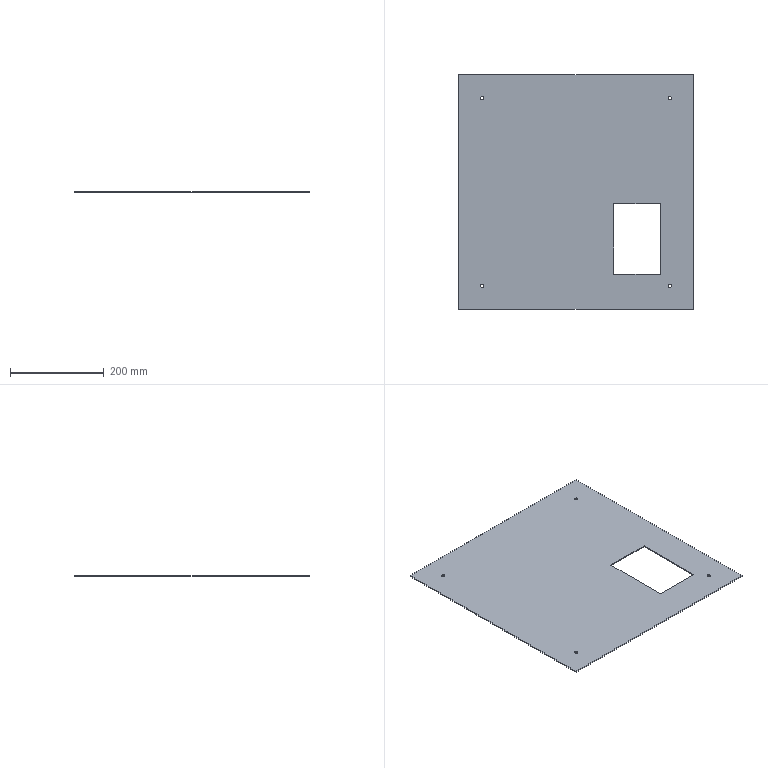Part | SolidWorks | features Extrusion 1, HoleWzd 1, ICE 1 | 1 solid | 18 faces | box 500 x 500 x 2 mm | volume 469692 mm3 | plane 10 | cylinder 8 | commonest cylinder face diameters 7 x8
STEP:
#1=CARTESIAN_POINT('',(-203.5,200.,0.));
#2=VERTEX_POINT('',#1);
#3=CARTESIAN_POINT('',(-196.5,200.,0.));
#4=VERTEX_POINT('',#3);
#5=CARTESIAN_POINT('',(-200.,200.,0.));
#6=DIRECTION('',(0.,0.,1.));
#7=DIRECTION('',(1.,0.,0.));
#8=AXIS2_PLACEMENT_3D('',#5,#6,#7);
#9=CIRCLE('',#8,3.5);
#10=EDGE_CURVE('',#2,#4,#9,.T.);
#11=ORIENTED_EDGE('',*,*,#10,.F.);
#12=CARTESIAN_POINT('',(-203.5,200.,2.));
#13=VERTEX_POINT('',#12);
#14=CARTESIAN_POINT('',(-203.5,200.,2.));
#15=DIRECTION('',(0.,0.,1.));
#16=VECTOR('',#15,1000.);
#17=LINE('',#14,#16);
#18=EDGE_CURVE('',#2,#13,#17,.T.);
#19=ORIENTED_EDGE('',*,*,#18,.T.);
#20=CARTESIAN_POINT('',(-196.5,200.,2.));
#21=VERTEX_POINT('',#20);
#22=CARTESIAN_POINT('',(-200.,200.,2.));
#23=DIRECTION('',(0.,0.,1.));
#24=DIRECTION('',(1.,0.,0.));
#25=AXIS2_PLACEMENT_3D('',#22,#23,#24);
#26=CIRCLE('',#25,3.5);
#27=EDGE_CURVE('',#13,#21,#26,.T.);
#28=ORIENTED_EDGE('',*,*,#27,.T.);
#29=CARTESIAN_POINT('',(-196.5,200.,2.));
#30=DIRECTION('',(0.,0.,1.));
#31=VECTOR('',#30,1000.);
#32=LINE('',#29,#31);
#33=EDGE_CURVE('',#4,#21,#32,.T.);
#34=ORIENTED_EDGE('',*,*,#33,.F.);
#35=EDGE_LOOP('',(#11,#19,#28,#34));
#36=FACE_OUTER_BOUND('',#35,.T.);
#37=CARTESIAN_POINT('',(-200.,200.,2.));
#38=DIRECTION('',(0.,0.,1.));
#39=DIRECTION('',(1.,0.,0.));
#40=AXIS2_PLACEMENT_3D('',#37,#38,#39);
#41=CYLINDRICAL_SURFACE('',#40,3.5);
#42=ADVANCED_FACE('',(#36),#41,.F.);
#43=CARTESIAN_POINT('',(196.5,200.,0.));
#44=VERTEX_POINT('',#43);
#45=CARTESIAN_POINT('',(203.5,200.,0.));
#46=VERTEX_POINT('',#45);
#47=CARTESIAN_POINT('',(200.,200.,0.));
#48=DIRECTION('',(0.,0.,1.));
#49=DIRECTION('',(1.,0.,0.));
#50=AXIS2_PLACEMENT_3D('',#47,#48,#49);
#51=CIRCLE('',#50,3.5);
#52=EDGE_CURVE('',#44,#46,#51,.T.);
#53=ORIENTED_EDGE('',*,*,#52,.F.);
#54=CARTESIAN_POINT('',(196.5,200.,2.));
#55=VERTEX_POINT('',#54);
#56=CARTESIAN_POINT('',(196.5,200.,2.));
#57=DIRECTION('',(0.,0.,1.));
#58=VECTOR('',#57,1000.);
#59=LINE('',#56,#58);
#60=EDGE_CURVE('',#44,#55,#59,.T.);
#61=ORIENTED_EDGE('',*,*,#60,.T.);
#62=CARTESIAN_POINT('',(203.5,200.,2.));
#63=VERTEX_POINT('',#62);
#64=CARTESIAN_POINT('',(200.,200.,2.));
#65=DIRECTION('',(0.,0.,1.));
#66=DIRECTION('',(1.,0.,0.));
#67=AXIS2_PLACEMENT_3D('',#64,#65,#66);
#68=CIRCLE('',#67,3.5);
#69=EDGE_CURVE('',#55,#63,#68,.T.);
#70=ORIENTED_EDGE('',*,*,#69,.T.);
#71=CARTESIAN_POINT('',(203.5,200.,2.));
#72=DIRECTION('',(0.,0.,1.));
#73=VECTOR('',#72,1000.);
#74=LINE('',#71,#73);
#75=EDGE_CURVE('',#46,#63,#74,.T.);
#76=ORIENTED_EDGE('',*,*,#75,.F.);
#77=EDGE_LOOP('',(#53,#61,#70,#76));
#78=FACE_OUTER_BOUND('',#77,.T.);
#79=CARTESIAN_POINT('',(200.,200.,2.));
#80=DIRECTION('',(0.,0.,1.));
#81=DIRECTION('',(1.,0.,0.));
#82=AXIS2_PLACEMENT_3D('',#79,#80,#81);
#83=CYLINDRICAL_SURFACE('',#82,3.5);
#84=ADVANCED_FACE('',(#78),#83,.F.);
#85=CARTESIAN_POINT('',(-203.5,-200.,0.));
#86=VERTEX_POINT('',#85);
#87=CARTESIAN_POINT('',(-196.5,-200.,0.));
#88=VERTEX_POINT('',#87);
#89=CARTESIAN_POINT('',(-200.,-200.,0.));
#90=DIRECTION('',(0.,0.,1.));
#91=DIRECTION('',(1.,0.,0.));
#92=AXIS2_PLACEMENT_3D('',#89,#90,#91);
#93=CIRCLE('',#92,3.5);
#94=EDGE_CURVE('',#86,#88,#93,.T.);
#95=ORIENTED_EDGE('',*,*,#94,.F.);
#96=CARTESIAN_POINT('',(-203.5,-200.,2.));
#97=VERTEX_POINT('',#96);
#98=CARTESIAN_POINT('',(-203.5,-200.,2.));
#99=DIRECTION('',(0.,0.,1.));
#100=VECTOR('',#99,1000.);
#101=LINE('',#98,#100);
#102=EDGE_CURVE('',#86,#97,#101,.T.);
#103=ORIENTED_EDGE('',*,*,#102,.T.);
#104=CARTESIAN_POINT('',(-196.5,-200.,2.));
#105=VERTEX_POINT('',#104);
#106=CARTESIAN_POINT('',(-200.,-200.,2.));
#107=DIRECTION('',(0.,0.,1.));
#108=DIRECTION('',(1.,0.,0.));
#109=AXIS2_PLACEMENT_3D('',#106,#107,#108);
#110=CIRCLE('',#109,3.5);
#111=EDGE_CURVE('',#97,#105,#110,.T.);
#112=ORIENTED_EDGE('',*,*,#111,.T.);
#113=CARTESIAN_POINT('',(-196.5,-200.,2.));
#114=DIRECTION('',(0.,0.,1.));
#115=VECTOR('',#114,1000.);
#116=LINE('',#113,#115);
#117=EDGE_CURVE('',#88,#105,#116,.T.);
#118=ORIENTED_EDGE('',*,*,#117,.F.);
#119=EDGE_LOOP('',(#95,#103,#112,#118));
#120=FACE_OUTER_BOUND('',#119,.T.);
#121=CARTESIAN_POINT('',(-200.,-200.,2.));
#122=DIRECTION('',(0.,0.,1.));
#123=DIRECTION('',(1.,0.,0.));
#124=AXIS2_PLACEMENT_3D('',#121,#122,#123);
#125=CYLINDRICAL_SURFACE('',#124,3.5);
#126=ADVANCED_FACE('',(#120),#125,.F.);
#127=CARTESIAN_POINT('',(196.5,-200.,0.));
#128=VERTEX_POINT('',#127);
#129=CARTESIAN_POINT('',(203.5,-200.,0.));
#130=VERTEX_POINT('',#129);
#131=CARTESIAN_POINT('',(200.,-200.,0.));
#132=DIRECTION('',(0.,0.,1.));
#133=DIRECTION('',(1.,0.,0.));
#134=AXIS2_PLACEMENT_3D('',#131,#132,#133);
#135=CIRCLE('',#134,3.5);
#136=EDGE_CURVE('',#128,#130,#135,.T.);
#137=ORIENTED_EDGE('',*,*,#136,.F.);
#138=CARTESIAN_POINT('',(196.5,-200.,2.));
#139=VERTEX_POINT('',#138);
#140=CARTESIAN_POINT('',(196.5,-200.,2.));
#141=DIRECTION('',(0.,0.,1.));
#142=VECTOR('',#141,1000.);
#143=LINE('',#140,#142);
#144=EDGE_CURVE('',#128,#139,#143,.T.);
#145=ORIENTED_EDGE('',*,*,#144,.T.);
#146=CARTESIAN_POINT('',(203.5,-200.,2.));
#147=VERTEX_POINT('',#146);
#148=CARTESIAN_POINT('',(200.,-200.,2.));
#149=DIRECTION('',(0.,0.,1.));
#150=DIRECTION('',(1.,0.,0.));
#151=AXIS2_PLACEMENT_3D('',#148,#149,#150);
#152=CIRCLE('',#151,3.5);
#153=EDGE_CURVE('',#139,#147,#152,.T.);
#154=ORIENTED_EDGE('',*,*,#153,.T.);
#155=CARTESIAN_POINT('',(203.5,-200.,2.));
#156=DIRECTION('',(0.,0.,1.));
#157=VECTOR('',#156,1000.);
#158=LINE('',#155,#157);
#159=EDGE_CURVE('',#130,#147,#158,.T.);
#160=ORIENTED_EDGE('',*,*,#159,.F.);
#161=EDGE_LOOP('',(#137,#145,#154,#160));
#162=FACE_OUTER_BOUND('',#161,.T.);
#163=CARTESIAN_POINT('',(200.,-200.,2.));
#164=DIRECTION('',(0.,0.,1.));
#165=DIRECTION('',(1.,0.,0.));
#166=AXIS2_PLACEMENT_3D('',#163,#164,#165);
#167=CYLINDRICAL_SURFACE('',#166,3.5);
#168=ADVANCED_FACE('',(#162),#167,.F.);
#169=CARTESIAN_POINT('',(250.,-250.,0.));
#170=VERTEX_POINT('',#169);
#171=CARTESIAN_POINT('',(250.,250.,0.));
#172=VERTEX_POINT('',#171);
#173=CARTESIAN_POINT('',(250.,250.,0.));
#174=DIRECTION('',(0.,1.,0.));
#175=VECTOR('',#174,1000.);
#176=LINE('',#173,#175);
#177=EDGE_CURVE('',#170,#172,#176,.T.);
#178=ORIENTED_EDGE('',*,*,#177,.T.);
#179=CARTESIAN_POINT('',(250.,250.,2.));
#180=VERTEX_POINT('',#179);
#181=CARTESIAN_POINT('',(250.,250.,2.));
#182=DIRECTION('',(0.,0.,-1.));
#183=VECTOR('',#182,1000.);
#184=LINE('',#181,#183);
#185=EDGE_CURVE('',#180,#172,#184,.T.);
#186=ORIENTED_EDGE('',*,*,#185,.F.);
#187=CARTESIAN_POINT('',(250.,-250.,2.));
#188=VERTEX_POINT('',#187);
#189=CARTESIAN_POINT('',(250.,250.,2.));
#190=DIRECTION('',(0.,1.,0.));
#191=VECTOR('',#190,1000.);
#192=LINE('',#189,#191);
#193=EDGE_CURVE('',#188,#180,#192,.T.);
#194=ORIENTED_EDGE('',*,*,#193,.F.);
#195=CARTESIAN_POINT('',(250.,-250.,2.));
#196=DIRECTION('',(0.,0.,-1.));
#197=VECTOR('',#196,1000.);
#198=LINE('',#195,#197);
#199=EDGE_CURVE('',#188,#170,#198,.T.);
#200=ORIENTED_EDGE('',*,*,#199,.T.);
#201=EDGE_LOOP('',(#178,#186,#194,#200));
#202=FACE_OUTER_BOUND('',#201,.T.);
#203=CARTESIAN_POINT('',(250.,250.,2.));
#204=DIRECTION('',(-1.,0.,0.));
#205=DIRECTION('',(0.,-1.,0.));
#206=AXIS2_PLACEMENT_3D('',#203,#204,#205);
#207=PLANE('',#206);
#208=ADVANCED_FACE('',(#202),#207,.F.);
#209=CARTESIAN_POINT('',(-250.,250.,0.));
#210=VERTEX_POINT('',#209);
#211=CARTESIAN_POINT('',(-250.,250.,0.));
#212=DIRECTION('',(-1.,0.,0.));
#213=VECTOR('',#212,1000.);
#214=LINE('',#211,#213);
#215=EDGE_CURVE('',#172,#210,#214,.T.);
#216=ORIENTED_EDGE('',*,*,#215,.T.);
#217=CARTESIAN_POINT('',(-250.,250.,2.));
#218=VERTEX_POINT('',#217);
#219=CARTESIAN_POINT('',(-250.,250.,2.));
#220=DIRECTION('',(0.,0.,-1.));
#221=VECTOR('',#220,1000.);
#222=LINE('',#219,#221);
#223=EDGE_CURVE('',#218,#210,#222,.T.);
#224=ORIENTED_EDGE('',*,*,#223,.F.);
#225=CARTESIAN_POINT('',(-250.,250.,2.));
#226=DIRECTION('',(-1.,0.,0.));
#227=VECTOR('',#226,1000.);
#228=LINE('',#225,#227);
#229=EDGE_CURVE('',#180,#218,#228,.T.);
#230=ORIENTED_EDGE('',*,*,#229,.F.);
#231=ORIENTED_EDGE('',*,*,#185,.T.);
#232=EDGE_LOOP('',(#216,#224,#230,#231));
#233=FACE_OUTER_BOUND('',#232,.T.);
#234=CARTESIAN_POINT('',(-250.,250.,2.));
#235=DIRECTION('',(0.,-1.,0.));
#236=DIRECTION('',(0.,0.,-1.));
#237=AXIS2_PLACEMENT_3D('',#234,#235,#236);
#238=PLANE('',#237);
#239=ADVANCED_FACE('',(#233),#238,.F.);
#240=CARTESIAN_POINT('',(-250.,-250.,0.));
#241=VERTEX_POINT('',#240);
#242=CARTESIAN_POINT('',(-250.,250.,0.));
#243=DIRECTION('',(0.,-1.,0.));
#244=VECTOR('',#243,1000.);
#245=LINE('',#242,#244);
#246=EDGE_CURVE('',#210,#241,#245,.T.);
#247=ORIENTED_EDGE('',*,*,#246,.T.);
#248=CARTESIAN_POINT('',(-250.,-250.,2.));
#249=VERTEX_POINT('',#248);
#250=CARTESIAN_POINT('',(-250.,-250.,2.));
#251=DIRECTION('',(0.,0.,-1.));
#252=VECTOR('',#251,1000.);
#253=LINE('',#250,#252);
#254=EDGE_CURVE('',#249,#241,#253,.T.);
#255=ORIENTED_EDGE('',*,*,#254,.F.);
#256=CARTESIAN_POINT('',(-250.,250.,2.));
#257=DIRECTION('',(0.,-1.,0.));
#258=VECTOR('',#257,1000.);
#259=LINE('',#256,#258);
#260=EDGE_CURVE('',#218,#249,#259,.T.);
#261=ORIENTED_EDGE('',*,*,#260,.F.);
#262=ORIENTED_EDGE('',*,*,#223,.T.);
#263=EDGE_LOOP('',(#247,#255,#261,#262));
#264=FACE_OUTER_BOUND('',#263,.T.);
#265=CARTESIAN_POINT('',(-250.,250.,2.));
#266=DIRECTION('',(1.,0.,0.));
#267=DIRECTION('',(0.,1.,0.));
#268=AXIS2_PLACEMENT_3D('',#265,#266,#267);
#269=PLANE('',#268);
#270=ADVANCED_FACE('',(#264),#269,.F.);
#271=CARTESIAN_POINT('',(-250.,-250.,0.));
#272=DIRECTION('',(1.,0.,0.));
#273=VECTOR('',#272,1000.);
#274=LINE('',#271,#273);
#275=EDGE_CURVE('',#241,#170,#274,.T.);
#276=ORIENTED_EDGE('',*,*,#275,.T.);
#277=ORIENTED_EDGE('',*,*,#199,.F.);
#278=CARTESIAN_POINT('',(-250.,-250.,2.));
#279=DIRECTION('',(1.,0.,0.));
#280=VECTOR('',#279,1000.);
#281=LINE('',#278,#280);
#282=EDGE_CURVE('',#249,#188,#281,.T.);
#283=ORIENTED_EDGE('',*,*,#282,.F.);
#284=ORIENTED_EDGE('',*,*,#254,.T.);
#285=EDGE_LOOP('',(#276,#277,#283,#284));
#286=FACE_OUTER_BOUND('',#285,.T.);
#287=CARTESIAN_POINT('',(-250.,-250.,2.));
#288=DIRECTION('',(0.,1.,0.));
#289=DIRECTION('',(0.,0.,1.));
#290=AXIS2_PLACEMENT_3D('',#287,#288,#289);
#291=PLANE('',#290);
#292=ADVANCED_FACE('',(#286),#291,.F.);
#293=CARTESIAN_POINT('',(180.,-175.,2.));
#294=VERTEX_POINT('',#293);
#295=CARTESIAN_POINT('',(180.,-25.,2.));
#296=VERTEX_POINT('',#295);
#297=CARTESIAN_POINT('',(180.,-25.,2.));
#298=DIRECTION('',(0.,1.,0.));
#299=VECTOR('',#298,1000.);
#300=LINE('',#297,#299);
#301=EDGE_CURVE('',#294,#296,#300,.T.);
#302=ORIENTED_EDGE('',*,*,#301,.F.);
#303=CARTESIAN_POINT('',(80.,-175.,2.));
#304=VERTEX_POINT('',#303);
#305=CARTESIAN_POINT('',(80.,-175.,2.));
#306=DIRECTION('',(1.,0.,0.));
#307=VECTOR('',#306,1000.);
#308=LINE('',#305,#307);
#309=EDGE_CURVE('',#304,#294,#308,.T.);
#310=ORIENTED_EDGE('',*,*,#309,.F.);
#311=CARTESIAN_POINT('',(80.,-25.,2.));
#312=VERTEX_POINT('',#311);
#313=CARTESIAN_POINT('',(80.,-25.,2.));
#314=DIRECTION('',(0.,-1.,0.));
#315=VECTOR('',#314,1000.);
#316=LINE('',#313,#315);
#317=EDGE_CURVE('',#312,#304,#316,.T.);
#318=ORIENTED_EDGE('',*,*,#317,.F.);
#319=CARTESIAN_POINT('',(80.,-25.,2.));
#320=DIRECTION('',(-1.,0.,0.));
#321=VECTOR('',#320,1000.);
#322=LINE('',#319,#321);
#323=EDGE_CURVE('',#296,#312,#322,.T.);
#324=ORIENTED_EDGE('',*,*,#323,.F.);
#325=EDGE_LOOP('',(#302,#310,#318,#324));
#326=FACE_BOUND('',#325,.T.);
#327=CARTESIAN_POINT('',(-200.,200.,2.));
#328=DIRECTION('',(0.,0.,1.));
#329=DIRECTION('',(1.,0.,0.));
#330=AXIS2_PLACEMENT_3D('',#327,#328,#329);
#331=CIRCLE('',#330,3.5);
#332=EDGE_CURVE('',#21,#13,#331,.T.);
#333=ORIENTED_EDGE('',*,*,#332,.F.);
#334=ORIENTED_EDGE('',*,*,#27,.F.);
#335=EDGE_LOOP('',(#333,#334));
#336=FACE_BOUND('',#335,.T.);
#337=CARTESIAN_POINT('',(200.,200.,2.));
#338=DIRECTION('',(0.,0.,1.));
#339=DIRECTION('',(1.,0.,0.));
#340=AXIS2_PLACEMENT_3D('',#337,#338,#339);
#341=CIRCLE('',#340,3.5);
#342=EDGE_CURVE('',#63,#55,#341,.T.);
#343=ORIENTED_EDGE('',*,*,#342,.F.);
#344=ORIENTED_EDGE('',*,*,#69,.F.);
#345=EDGE_LOOP('',(#343,#344));
#346=FACE_BOUND('',#345,.T.);
#347=CARTESIAN_POINT('',(-200.,-200.,2.));
#348=DIRECTION('',(0.,0.,1.));
#349=DIRECTION('',(1.,0.,0.));
#350=AXIS2_PLACEMENT_3D('',#347,#348,#349);
#351=CIRCLE('',#350,3.5);
#352=EDGE_CURVE('',#105,#97,#351,.T.);
#353=ORIENTED_EDGE('',*,*,#352,.F.);
#354=ORIENTED_EDGE('',*,*,#111,.F.);
#355=EDGE_LOOP('',(#353,#354));
#356=FACE_BOUND('',#355,.T.);
#357=CARTESIAN_POINT('',(200.,-200.,2.));
#358=DIRECTION('',(0.,0.,1.));
#359=DIRECTION('',(1.,0.,0.));
#360=AXIS2_PLACEMENT_3D('',#357,#358,#359);
#361=CIRCLE('',#360,3.5);
#362=EDGE_CURVE('',#147,#139,#361,.T.);
#363=ORIENTED_EDGE('',*,*,#362,.F.);
#364=ORIENTED_EDGE('',*,*,#153,.F.);
#365=EDGE_LOOP('',(#363,#364));
#366=FACE_BOUND('',#365,.T.);
#367=ORIENTED_EDGE('',*,*,#193,.T.);
#368=ORIENTED_EDGE('',*,*,#229,.T.);
#369=ORIENTED_EDGE('',*,*,#260,.T.);
#370=ORIENTED_EDGE('',*,*,#282,.T.);
#371=EDGE_LOOP('',(#367,#368,#369,#370));
#372=FACE_OUTER_BOUND('',#371,.T.);
#373=CARTESIAN_POINT('',(0.,0.,2.));
#374=DIRECTION('',(0.,0.,1.));
#375=DIRECTION('',(1.,0.,0.));
#376=AXIS2_PLACEMENT_3D('',#373,#374,#375);
#377=PLANE('',#376);
#378=ADVANCED_FACE('',(#326,#336,#346,#356,#366,#372),#377,.T.);
#379=CARTESIAN_POINT('',(80.,-175.,0.));
#380=VERTEX_POINT('',#379);
#381=CARTESIAN_POINT('',(180.,-175.,0.));
#382=VERTEX_POINT('',#381);
#383=CARTESIAN_POINT('',(80.,-175.,0.));
#384=DIRECTION('',(1.,0.,0.));
#385=VECTOR('',#384,1000.);
#386=LINE('',#383,#385);
#387=EDGE_CURVE('',#380,#382,#386,.T.);
#388=ORIENTED_EDGE('',*,*,#387,.T.);
#389=CARTESIAN_POINT('',(180.,-25.,0.));
#390=VERTEX_POINT('',#389);
#391=CARTESIAN_POINT('',(180.,-25.,0.));
#392=DIRECTION('',(0.,1.,0.));
#393=VECTOR('',#392,1000.);
#394=LINE('',#391,#393);
#395=EDGE_CURVE('',#382,#390,#394,.T.);
#396=ORIENTED_EDGE('',*,*,#395,.T.);
#397=CARTESIAN_POINT('',(80.,-25.,0.));
#398=VERTEX_POINT('',#397);
#399=CARTESIAN_POINT('',(80.,-25.,0.));
#400=DIRECTION('',(-1.,0.,0.));
#401=VECTOR('',#400,1000.);
#402=LINE('',#399,#401);
#403=EDGE_CURVE('',#390,#398,#402,.T.);
#404=ORIENTED_EDGE('',*,*,#403,.T.);
#405=CARTESIAN_POINT('',(80.,-25.,0.));
#406=DIRECTION('',(0.,-1.,0.));
#407=VECTOR('',#406,1000.);
#408=LINE('',#405,#407);
#409=EDGE_CURVE('',#398,#380,#408,.T.);
#410=ORIENTED_EDGE('',*,*,#409,.T.);
#411=EDGE_LOOP('',(#388,#396,#404,#410));
#412=FACE_BOUND('',#411,.T.);
#413=CARTESIAN_POINT('',(-200.,200.,0.));
#414=DIRECTION('',(0.,0.,1.));
#415=DIRECTION('',(1.,0.,0.));
#416=AXIS2_PLACEMENT_3D('',#413,#414,#415);
#417=CIRCLE('',#416,3.5);
#418=EDGE_CURVE('',#4,#2,#417,.T.);
#419=ORIENTED_EDGE('',*,*,#418,.T.);
#420=ORIENTED_EDGE('',*,*,#10,.T.);
#421=EDGE_LOOP('',(#419,#420));
#422=FACE_BOUND('',#421,.T.);
#423=CARTESIAN_POINT('',(200.,200.,0.));
#424=DIRECTION('',(0.,0.,1.));
#425=DIRECTION('',(1.,0.,0.));
#426=AXIS2_PLACEMENT_3D('',#423,#424,#425);
#427=CIRCLE('',#426,3.5);
#428=EDGE_CURVE('',#46,#44,#427,.T.);
#429=ORIENTED_EDGE('',*,*,#428,.T.);
#430=ORIENTED_EDGE('',*,*,#52,.T.);
#431=EDGE_LOOP('',(#429,#430));
#432=FACE_BOUND('',#431,.T.);
#433=CARTESIAN_POINT('',(-200.,-200.,0.));
#434=DIRECTION('',(0.,0.,1.));
#435=DIRECTION('',(1.,0.,0.));
#436=AXIS2_PLACEMENT_3D('',#433,#434,#435);
#437=CIRCLE('',#436,3.5);
#438=EDGE_CURVE('',#88,#86,#437,.T.);
#439=ORIENTED_EDGE('',*,*,#438,.T.);
#440=ORIENTED_EDGE('',*,*,#94,.T.);
#441=EDGE_LOOP('',(#439,#440));
#442=FACE_BOUND('',#441,.T.);
#443=CARTESIAN_POINT('',(200.,-200.,0.));
#444=DIRECTION('',(0.,0.,1.));
#445=DIRECTION('',(1.,0.,0.));
#446=AXIS2_PLACEMENT_3D('',#443,#444,#445);
#447=CIRCLE('',#446,3.5);
#448=EDGE_CURVE('',#130,#128,#447,.T.);
#449=ORIENTED_EDGE('',*,*,#448,.T.);
#450=ORIENTED_EDGE('',*,*,#136,.T.);
#451=EDGE_LOOP('',(#449,#450));
#452=FACE_BOUND('',#451,.T.);
#453=ORIENTED_EDGE('',*,*,#177,.F.);
#454=ORIENTED_EDGE('',*,*,#275,.F.);
#455=ORIENTED_EDGE('',*,*,#246,.F.);
#456=ORIENTED_EDGE('',*,*,#215,.F.);
#457=EDGE_LOOP('',(#453,#454,#455,#456));
#458=FACE_OUTER_BOUND('',#457,.T.);
#459=CARTESIAN_POINT('',(0.,0.,0.));
#460=DIRECTION('',(0.,0.,1.));
#461=DIRECTION('',(1.,0.,0.));
#462=AXIS2_PLACEMENT_3D('',#459,#460,#461);
#463=PLANE('',#462);
#464=ADVANCED_FACE('',(#412,#422,#432,#442,#452,#458),#463,.F.);
#465=ORIENTED_EDGE('',*,*,#144,.F.);
#466=ORIENTED_EDGE('',*,*,#448,.F.);
#467=ORIENTED_EDGE('',*,*,#159,.T.);
#468=ORIENTED_EDGE('',*,*,#362,.T.);
#469=EDGE_LOOP('',(#465,#466,#467,#468));
#470=FACE_OUTER_BOUND('',#469,.T.);
#471=CARTESIAN_POINT('',(200.,-200.,2.));
#472=DIRECTION('',(0.,0.,1.));
#473=DIRECTION('',(1.,0.,0.));
#474=AXIS2_PLACEMENT_3D('',#471,#472,#473);
#475=CYLINDRICAL_SURFACE('',#474,3.5);
#476=ADVANCED_FACE('',(#470),#475,.F.);
#477=ORIENTED_EDGE('',*,*,#102,.F.);
#478=ORIENTED_EDGE('',*,*,#438,.F.);
#479=ORIENTED_EDGE('',*,*,#117,.T.);
#480=ORIENTED_EDGE('',*,*,#352,.T.);
#481=EDGE_LOOP('',(#477,#478,#479,#480));
#482=FACE_OUTER_BOUND('',#481,.T.);
#483=CARTESIAN_POINT('',(-200.,-200.,2.));
#484=DIRECTION('',(0.,0.,1.));
#485=DIRECTION('',(1.,0.,0.));
#486=AXIS2_PLACEMENT_3D('',#483,#484,#485);
#487=CYLINDRICAL_SURFACE('',#486,3.5);
#488=ADVANCED_FACE('',(#482),#487,.F.);
#489=ORIENTED_EDGE('',*,*,#60,.F.);
#490=ORIENTED_EDGE('',*,*,#428,.F.);
#491=ORIENTED_EDGE('',*,*,#75,.T.);
#492=ORIENTED_EDGE('',*,*,#342,.T.);
#493=EDGE_LOOP('',(#489,#490,#491,#492));
#494=FACE_OUTER_BOUND('',#493,.T.);
#495=CARTESIAN_POINT('',(200.,200.,2.));
#496=DIRECTION('',(0.,0.,1.));
#497=DIRECTION('',(1.,0.,0.));
#498=AXIS2_PLACEMENT_3D('',#495,#496,#497);
#499=CYLINDRICAL_SURFACE('',#498,3.5);
#500=ADVANCED_FACE('',(#494),#499,.F.);
#501=ORIENTED_EDGE('',*,*,#18,.F.);
#502=ORIENTED_EDGE('',*,*,#418,.F.);
#503=ORIENTED_EDGE('',*,*,#33,.T.);
#504=ORIENTED_EDGE('',*,*,#332,.T.);
#505=EDGE_LOOP('',(#501,#502,#503,#504));
#506=FACE_OUTER_BOUND('',#505,.T.);
#507=CARTESIAN_POINT('',(-200.,200.,2.));
#508=DIRECTION('',(0.,0.,1.));
#509=DIRECTION('',(1.,0.,0.));
#510=AXIS2_PLACEMENT_3D('',#507,#508,#509);
#511=CYLINDRICAL_SURFACE('',#510,3.5);
#512=ADVANCED_FACE('',(#506),#511,.F.);
#513=ORIENTED_EDGE('',*,*,#301,.T.);
#514=CARTESIAN_POINT('',(180.,-25.,0.));
#515=DIRECTION('',(0.,0.,1.));
#516=VECTOR('',#515,1000.);
#517=LINE('',#514,#516);
#518=EDGE_CURVE('',#390,#296,#517,.T.);
#519=ORIENTED_EDGE('',*,*,#518,.F.);
#520=ORIENTED_EDGE('',*,*,#395,.F.);
#521=CARTESIAN_POINT('',(180.,-175.,0.));
#522=DIRECTION('',(0.,0.,1.));
#523=VECTOR('',#522,1000.);
#524=LINE('',#521,#523);
#525=EDGE_CURVE('',#382,#294,#524,.T.);
#526=ORIENTED_EDGE('',*,*,#525,.T.);
#527=EDGE_LOOP('',(#513,#519,#520,#526));
#528=FACE_OUTER_BOUND('',#527,.T.);
#529=CARTESIAN_POINT('',(180.,-25.,0.));
#530=DIRECTION('',(1.,0.,0.));
#531=DIRECTION('',(0.,1.,0.));
#532=AXIS2_PLACEMENT_3D('',#529,#530,#531);
#533=PLANE('',#532);
#534=ADVANCED_FACE('',(#528),#533,.F.);
#535=ORIENTED_EDGE('',*,*,#309,.T.);
#536=ORIENTED_EDGE('',*,*,#525,.F.);
#537=ORIENTED_EDGE('',*,*,#387,.F.);
#538=CARTESIAN_POINT('',(80.,-175.,0.));
#539=DIRECTION('',(0.,0.,1.));
#540=VECTOR('',#539,1000.);
#541=LINE('',#538,#540);
#542=EDGE_CURVE('',#380,#304,#541,.T.);
#543=ORIENTED_EDGE('',*,*,#542,.T.);
#544=EDGE_LOOP('',(#535,#536,#537,#543));
#545=FACE_OUTER_BOUND('',#544,.T.);
#546=CARTESIAN_POINT('',(80.,-175.,0.));
#547=DIRECTION('',(0.,-1.,0.));
#548=DIRECTION('',(0.,0.,-1.));
#549=AXIS2_PLACEMENT_3D('',#546,#547,#548);
#550=PLANE('',#549);
#551=ADVANCED_FACE('',(#545),#550,.F.);
#552=ORIENTED_EDGE('',*,*,#317,.T.);
#553=ORIENTED_EDGE('',*,*,#542,.F.);
#554=ORIENTED_EDGE('',*,*,#409,.F.);
#555=CARTESIAN_POINT('',(80.,-25.,0.));
#556=DIRECTION('',(0.,0.,1.));
#557=VECTOR('',#556,1000.);
#558=LINE('',#555,#557);
#559=EDGE_CURVE('',#398,#312,#558,.T.);
#560=ORIENTED_EDGE('',*,*,#559,.T.);
#561=EDGE_LOOP('',(#552,#553,#554,#560));
#562=FACE_OUTER_BOUND('',#561,.T.);
#563=CARTESIAN_POINT('',(80.,-25.,0.));
#564=DIRECTION('',(-1.,0.,0.));
#565=DIRECTION('',(0.,-1.,0.));
#566=AXIS2_PLACEMENT_3D('',#563,#564,#565);
#567=PLANE('',#566);
#568=ADVANCED_FACE('',(#562),#567,.F.);
#569=ORIENTED_EDGE('',*,*,#323,.T.);
#570=ORIENTED_EDGE('',*,*,#559,.F.);
#571=ORIENTED_EDGE('',*,*,#403,.F.);
#572=ORIENTED_EDGE('',*,*,#518,.T.);
#573=EDGE_LOOP('',(#569,#570,#571,#572));
#574=FACE_OUTER_BOUND('',#573,.T.);
#575=CARTESIAN_POINT('',(80.,-25.,0.));
#576=DIRECTION('',(0.,1.,0.));
#577=DIRECTION('',(0.,0.,1.));
#578=AXIS2_PLACEMENT_3D('',#575,#576,#577);
#579=PLANE('',#578);
#580=ADVANCED_FACE('',(#574),#579,.F.);
#581=CLOSED_SHELL('',(#42,#84,#126,#168,#208,#239,#270,#292,#378,#464,#476,#488,#500,#512,#534,#551,#568,#580));
#582=MANIFOLD_SOLID_BREP('',#581);
#583=CARTESIAN_POINT('',(0.,0.,0.));
#584=DIRECTION('',(0.,0.,1.));
#585=DIRECTION('',(1.,0.,0.));
#586=AXIS2_PLACEMENT_3D('',#583,#584,#585);
#587=(LENGTH_UNIT()NAMED_UNIT(*)SI_UNIT(.MILLI.,.METRE.));
#588=UNCERTAINTY_MEASURE_WITH_UNIT(LENGTH_MEASURE(0.00001),#587,'','');
#589=(NAMED_UNIT(*)PLANE_ANGLE_UNIT()SI_UNIT($,.RADIAN.));
#590=(NAMED_UNIT(*)SI_UNIT($,.STERADIAN.)SOLID_ANGLE_UNIT());
#591=(GEOMETRIC_REPRESENTATION_CONTEXT(3)GLOBAL_UNCERTAINTY_ASSIGNED_CONTEXT((#588))GLOBAL_UNIT_ASSIGNED_CONTEXT((#587,#589,#590))REPRESENTATION_CONTEXT('',''));
#592=ADVANCED_BREP_SHAPE_REPRESENTATION('',(#582,#586),#591);